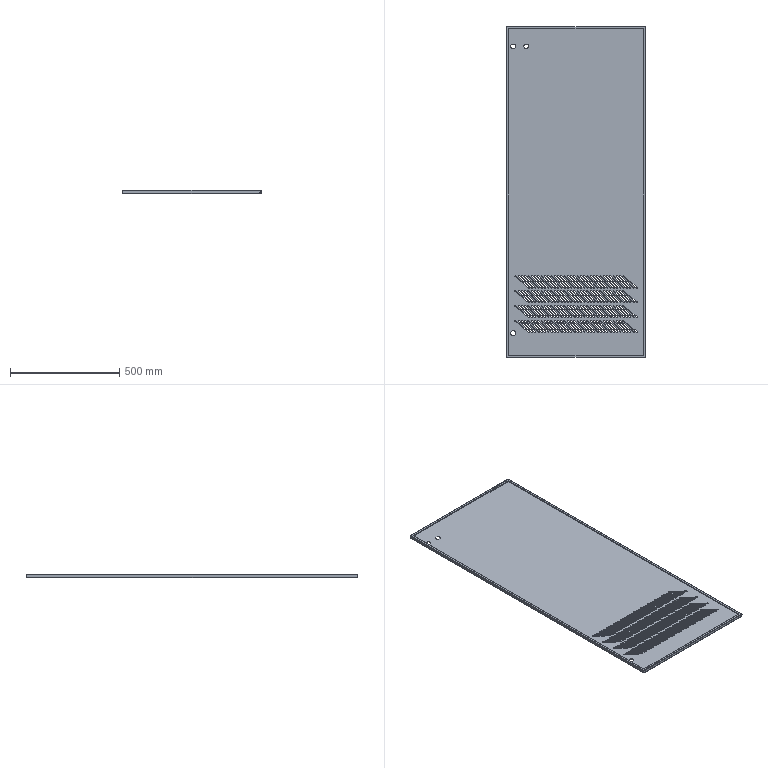Part | STEP file | HESS-408-70-15W-D-5-electrical box door panel | 1 solid | 783 faces | box 636 x 1516 x 14 mm | volume 1489085 mm3 | cylinder 439 | plane 328 | spline 16 | commonest cylinder face diameters 5 x412 0.2 x8 3.2 x8 22.5 x8 22 x3